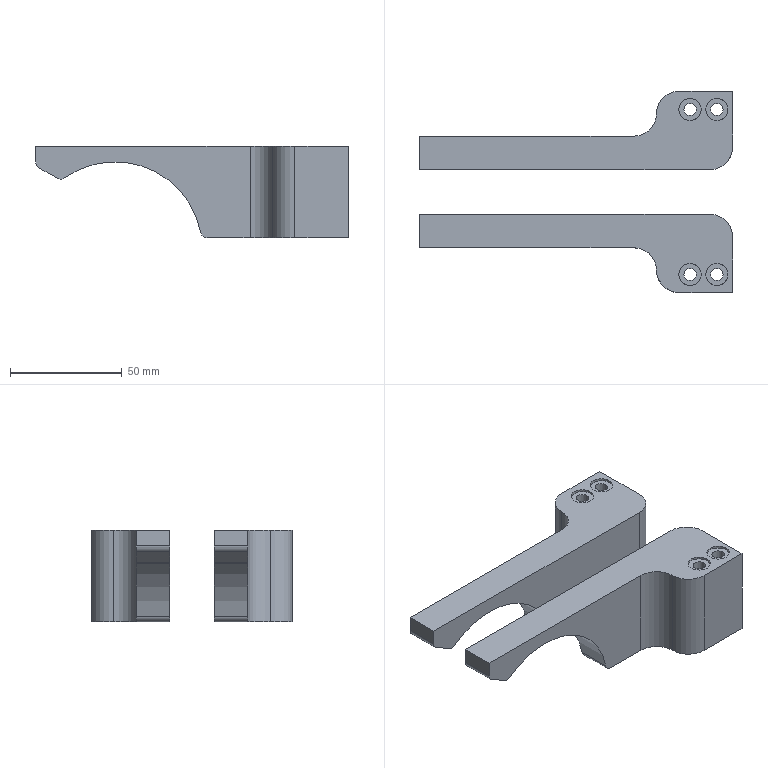NC program | NX | posted with a generic post | part box 140 x 90 x 41 mm
Lines 1 to 42 of 28919:
N10 G17 G21 G94 G90
(FLOOR_WALL , TOOL : D63)
N12 T01 M6
N14 G54
N16 G17 G0 G90 X109.5 Y0. S6500 M3
N18 G43 Z30. H1
N20 Z3.
N22 G94 G1 Z0. F1500.
N24 X106.5
N26 X-106.5
N28 X-109.5
N30 Z3.
N32 G0 Z30.
N34 M5
(DRILLING , TOOL : D6A45)
N36 T07 M6
N38 G54
N40 G17 G0 G90 X51.003 Y9.4 S5000 M3
N42 G43 Z30. H7
N44 G94 G81 G98 Z-1. F250. R3.
N46 X63.003
N48 G80
N50 G0 X63.003 Y9.4 Z30.
N52 M5
(DRILLING_COPY , TOOL : 5.5ZT)
N54 T15 M6
N56 G54
N58 G17 G0 G90 X51.003 Y9.4 S2000 M3
N60 G43 Z30. H15
N62 G94 G83 G98 Z-42.652 F200. Q2. R3.
N64 X63.003
N66 G80
N68 G0 X63.003 Y9.4 Z30.
N70 M5